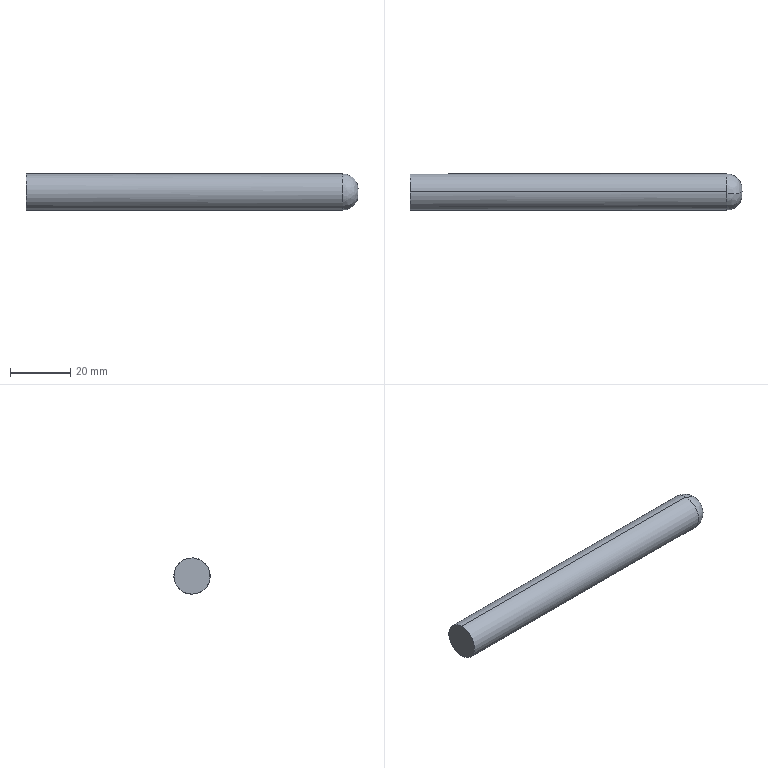Part | Creo | 1 solid | 6 faces | box 109.947 x 12 x 12 mm | volume 12270 mm3 | plane 2 | cylinder 2 | spline 2 | commonest cylinder face diameters 12 x2
STEP:
#1=CARTESIAN_POINT('',(0.,0.,0.));
#2=DIRECTION('',(0.,0.,1.));
#3=DIRECTION('',(1.,0.,0.));
#4=AXIS2_PLACEMENT_3D('',#1,#2,#3);
#5=CARTESIAN_POINT('',(51.36,96.983,-27.835));
#6=VERTEX_POINT('',#5);
#7=CARTESIAN_POINT('',(51.36,96.983,-39.835));
#8=VERTEX_POINT('',#7);
#9=CARTESIAN_POINT('',(51.36,96.983,-33.835));
#10=DIRECTION('',(-1.,0.,0.000000164));
#11=DIRECTION('',(0.000000164,0.,1.));
#12=AXIS2_PLACEMENT_3D('',#9,#10,#11);
#13=CIRCLE('',#12,6.);
#14=EDGE_CURVE('',#6,#8,#13,.T.);
#15=ORIENTED_EDGE('',*,*,#14,.F.);
#16=CARTESIAN_POINT('',(51.36,95.729,-27.968));
#17=VERTEX_POINT('',#16);
#18=CARTESIAN_POINT('',(51.36,96.983,-33.835));
#19=DIRECTION('',(-1.,0.,0.000000164));
#20=DIRECTION('',(0.000000161,-0.209,0.9779));
#21=AXIS2_PLACEMENT_3D('',#18,#19,#20);
#22=CIRCLE('',#21,6.);
#23=EDGE_CURVE('',#17,#6,#22,.T.);
#24=ORIENTED_EDGE('',*,*,#23,.F.);
#25=CARTESIAN_POINT('',(51.36,96.983,-33.835));
#26=DIRECTION('',(-1.,0.,0.000000164));
#27=DIRECTION('',(-0.000000164,0.,-1.));
#28=AXIS2_PLACEMENT_3D('',#25,#26,#27);
#29=CIRCLE('',#28,6.);
#30=EDGE_CURVE('',#8,#17,#29,.T.);
#31=ORIENTED_EDGE('',*,*,#30,.F.);
#32=EDGE_LOOP('',(#15,#24,#31));
#33=FACE_OUTER_BOUND('',#32,.F.);
#34=CARTESIAN_POINT('',(51.36,96.983,-33.835));
#35=DIRECTION('',(-1.,0.,0.000000197));
#36=DIRECTION('',(0.000000197,0.,1.));
#37=AXIS2_PLACEMENT_3D('',#34,#35,#36);
#38=PLANE('',#37);
#39=ADVANCED_FACE('',(#33),#38,.T.);
#40=CARTESIAN_POINT('',(156.307,97.613,-39.802));
#41=VERTEX_POINT('',#40);
#42=CARTESIAN_POINT('',(156.307,96.983,-27.835));
#43=VERTEX_POINT('',#42);
#44=CARTESIAN_POINT('',(156.307,96.983,-33.835));
#45=DIRECTION('',(1.,0.,-0.000000164));
#46=DIRECTION('',(-0.000000164,0.1051,-0.9945));
#47=AXIS2_PLACEMENT_3D('',#44,#45,#46);
#48=CIRCLE('',#47,6.);
#49=EDGE_CURVE('',#41,#43,#48,.T.);
#50=ORIENTED_EDGE('',*,*,#49,.T.);
#51=CARTESIAN_POINT('',(156.307,96.983,-27.835));
#52=DIRECTION('',(-1.,0.000001829,0.00000016));
#53=VECTOR('',#52,104.947);
#54=LINE('',#51,#53);
#55=EDGE_CURVE('',#43,#6,#54,.T.);
#56=ORIENTED_EDGE('',*,*,#55,.T.);
#57=ORIENTED_EDGE('',*,*,#14,.T.);
#58=CARTESIAN_POINT('',(156.307,96.983,-39.835));
#59=VERTEX_POINT('',#58);
#60=CARTESIAN_POINT('',(156.307,96.983,-39.835));
#61=DIRECTION('',(-1.,-0.000001503,0.000000164));
#62=VECTOR('',#61,104.947);
#63=LINE('',#60,#62);
#64=EDGE_CURVE('',#59,#8,#63,.T.);
#65=ORIENTED_EDGE('',*,*,#64,.F.);
#66=CARTESIAN_POINT('',(156.307,96.983,-33.835));
#67=DIRECTION('',(1.,0.,-0.000000164));
#68=DIRECTION('',(-0.000000164,0.,-1.));
#69=AXIS2_PLACEMENT_3D('',#66,#67,#68);
#70=CIRCLE('',#69,6.);
#71=EDGE_CURVE('',#59,#41,#70,.T.);
#72=ORIENTED_EDGE('',*,*,#71,.T.);
#73=EDGE_LOOP('',(#50,#56,#57,#65,#72));
#74=FACE_OUTER_BOUND('',#73,.F.);
#75=CARTESIAN_POINT('',(132.478,96.983,-33.835));
#76=DIRECTION('',(-1.,0.,0.000000164));
#77=DIRECTION('',(0.000000164,0.,1.));
#78=AXIS2_PLACEMENT_3D('',#75,#76,#77);
#79=CYLINDRICAL_SURFACE('',#78,6.);
#80=ADVANCED_FACE('',(#74),#79,.T.);
#81=ORIENTED_EDGE('',*,*,#49,.F.);
#82=CARTESIAN_POINT('',(161.307,97.088,-34.83));
#83=VERTEX_POINT('',#82);
#84=CARTESIAN_POINT('',(156.307,97.088,-34.83));
#85=DIRECTION('',(-0.000000017,-0.9945,-0.1051));
#86=DIRECTION('',(-0.000000164,0.1051,-0.9945));
#87=AXIS2_PLACEMENT_3D('',#84,#85,#86);
#88=CIRCLE('',#87,5.);
#89=EDGE_CURVE('',#41,#83,#88,.T.);
#90=ORIENTED_EDGE('',*,*,#89,.T.);
#91=CARTESIAN_POINT('',(161.307,96.878,-32.841));
#92=VERTEX_POINT('',#91);
#93=CARTESIAN_POINT('',(161.307,97.088,-34.83));
#94=CARTESIAN_POINT('',(161.307,97.197,-34.818));
#95=CARTESIAN_POINT('',(161.307,97.398,-34.763));
#96=CARTESIAN_POINT('',(161.307,97.667,-34.587));
#97=CARTESIAN_POINT('',(161.307,97.863,-34.343));
#98=CARTESIAN_POINT('',(161.307,97.977,-34.05));
#99=CARTESIAN_POINT('',(161.307,97.994,-33.732));
#100=CARTESIAN_POINT('',(161.307,97.913,-33.425));
#101=CARTESIAN_POINT('',(161.307,97.743,-33.16));
#102=CARTESIAN_POINT('',(161.307,97.499,-32.959));
#103=CARTESIAN_POINT('',(161.307,97.196,-32.841));
#104=CARTESIAN_POINT('',(161.307,96.987,-32.829));
#105=CARTESIAN_POINT('',(161.307,96.878,-32.841));
#106=B_SPLINE_CURVE_WITH_KNOTS('',3,(#93,#94,#95,#96,#97,#98,#99,#100,#101,#102,#103,#104,#105),.UNSPECIFIED.,.F.,.F.,(4,1,1,1,1,1,1,1,1,1,4),(0.,0.1,0.2,0.3,0.4,0.5,0.6,0.7,0.8,0.9,1.),.UNSPECIFIED.);
#107=EDGE_CURVE('',#83,#92,#106,.T.);
#108=ORIENTED_EDGE('',*,*,#107,.T.);
#109=CARTESIAN_POINT('',(156.307,96.353,-27.869));
#110=VERTEX_POINT('',#109);
#111=CARTESIAN_POINT('',(156.307,96.878,-32.841));
#112=DIRECTION('',(0.000000017,0.9945,0.1051));
#113=DIRECTION('',(0.000000164,-0.1051,0.9945));
#114=AXIS2_PLACEMENT_3D('',#111,#112,#113);
#115=CIRCLE('',#114,5.);
#116=EDGE_CURVE('',#110,#92,#115,.T.);
#117=ORIENTED_EDGE('',*,*,#116,.F.);
#118=CARTESIAN_POINT('',(156.307,96.983,-33.835));
#119=DIRECTION('',(1.,0.,-0.000000164));
#120=DIRECTION('',(0.000000164,0.,1.));
#121=AXIS2_PLACEMENT_3D('',#118,#119,#120);
#122=CIRCLE('',#121,6.);
#123=EDGE_CURVE('',#43,#110,#122,.T.);
#124=ORIENTED_EDGE('',*,*,#123,.F.);
#125=EDGE_LOOP('',(#81,#90,#108,#117,#124));
#126=FACE_OUTER_BOUND('',#125,.F.);
#127=CARTESIAN_POINT('',(156.15,96.813,-39.83));
#128=CARTESIAN_POINT('',(159.226,96.81,-39.927));
#129=CARTESIAN_POINT('',(161.402,96.872,-37.752));
#130=CARTESIAN_POINT('',(161.305,96.959,-34.677));
#131=CARTESIAN_POINT('',(156.15,100.709,-39.941));
#132=CARTESIAN_POINT('',(159.226,100.769,-40.039));
#133=CARTESIAN_POINT('',(161.402,99.417,-37.824));
#134=CARTESIAN_POINT('',(161.305,97.506,-34.692));
#135=CARTESIAN_POINT('',(156.15,103.357,-37.081));
#136=CARTESIAN_POINT('',(159.226,103.46,-37.133));
#137=CARTESIAN_POINT('',(161.402,101.147,-35.956));
#138=CARTESIAN_POINT('',(161.305,97.878,-34.291));
#139=CARTESIAN_POINT('',(156.15,102.947,-33.205));
#140=CARTESIAN_POINT('',(159.226,103.043,-33.195));
#141=CARTESIAN_POINT('',(161.402,100.879,-33.424));
#142=CARTESIAN_POINT('',(161.305,97.82,-33.747));
#143=CARTESIAN_POINT('',(156.15,102.538,-29.329));
#144=CARTESIAN_POINT('',(159.226,102.627,-29.256));
#145=CARTESIAN_POINT('',(161.402,100.612,-30.892));
#146=CARTESIAN_POINT('',(161.305,97.763,-33.203));
#147=CARTESIAN_POINT('',(156.15,99.351,-27.086));
#148=CARTESIAN_POINT('',(159.226,99.389,-26.977));
#149=CARTESIAN_POINT('',(161.402,98.53,-29.426));
#150=CARTESIAN_POINT('',(161.305,97.315,-32.888));
#151=CARTESIAN_POINT('',(156.15,95.564,-28.008));
#152=CARTESIAN_POINT('',(159.226,95.541,-27.914));
#153=CARTESIAN_POINT('',(161.402,96.056,-30.029));
#154=CARTESIAN_POINT('',(161.305,96.784,-33.017));
#155=(BOUNDED_SURFACE()B_SPLINE_SURFACE(3,3,((#127,#128,#129,#130),(#131,#132,#133,#134),(#135,#136,#137,#138),(#139,#140,#141,#142),(#143,#144,#145,#146),(#147,#148,#149,#150),(#151,#152,#153,#154)),.UNSPECIFIED.,.F.,.F.,.F.)B_SPLINE_SURFACE_WITH_KNOTS((4,3,4),(4,4),(0.,1.,2.),(0.,1.),.UNSPECIFIED.)GEOMETRIC_REPRESENTATION_ITEM()RATIONAL_B_SPLINE_SURFACE(((1.432,1.131,1.131,1.432),(1.106,0.8732,0.8732,1.106),(1.106,0.8732,0.8732,1.106),(1.432,1.131,1.131,1.432),(1.106,0.8732,0.8732,1.106),(1.106,0.8732,0.8732,1.106),(1.432,1.131,1.131,1.432)))REPRESENTATION_ITEM('')SURFACE());
#156=ADVANCED_FACE('',(#126),#155,.T.);
#157=CARTESIAN_POINT('',(156.307,96.983,-33.835));
#158=DIRECTION('',(1.,0.,-0.000000164));
#159=DIRECTION('',(0.000000164,-0.1051,0.9945));
#160=AXIS2_PLACEMENT_3D('',#157,#158,#159);
#161=CIRCLE('',#160,6.);
#162=EDGE_CURVE('',#110,#59,#161,.T.);
#163=ORIENTED_EDGE('',*,*,#162,.F.);
#164=ORIENTED_EDGE('',*,*,#116,.T.);
#165=CARTESIAN_POINT('',(161.307,96.878,-32.841));
#166=CARTESIAN_POINT('',(161.307,96.769,-32.852));
#167=CARTESIAN_POINT('',(161.307,96.568,-32.908));
#168=CARTESIAN_POINT('',(161.307,96.299,-33.083));
#169=CARTESIAN_POINT('',(161.307,96.103,-33.327));
#170=CARTESIAN_POINT('',(161.307,95.99,-33.621));
#171=CARTESIAN_POINT('',(161.307,95.972,-33.938));
#172=CARTESIAN_POINT('',(161.307,96.053,-34.245));
#173=CARTESIAN_POINT('',(161.307,96.224,-34.51));
#174=CARTESIAN_POINT('',(161.307,96.467,-34.712));
#175=CARTESIAN_POINT('',(161.307,96.77,-34.829));
#176=CARTESIAN_POINT('',(161.307,96.979,-34.841));
#177=CARTESIAN_POINT('',(161.307,97.088,-34.83));
#178=B_SPLINE_CURVE_WITH_KNOTS('',3,(#165,#166,#167,#168,#169,#170,#171,#172,#173,#174,#175,#176,#177),.UNSPECIFIED.,.F.,.F.,(4,1,1,1,1,1,1,1,1,1,4),(0.,0.1,0.2,0.3,0.4,0.5,0.6,0.7,0.8,0.9,1.),.UNSPECIFIED.);
#179=EDGE_CURVE('',#92,#83,#178,.T.);
#180=ORIENTED_EDGE('',*,*,#179,.T.);
#181=ORIENTED_EDGE('',*,*,#89,.F.);
#182=ORIENTED_EDGE('',*,*,#71,.F.);
#183=EDGE_LOOP('',(#163,#164,#180,#181,#182));
#184=FACE_OUTER_BOUND('',#183,.F.);
#185=CARTESIAN_POINT('',(156.15,97.153,-27.84));
#186=CARTESIAN_POINT('',(159.226,97.156,-27.744));
#187=CARTESIAN_POINT('',(161.402,97.094,-29.919));
#188=CARTESIAN_POINT('',(161.305,97.007,-32.994));
#189=CARTESIAN_POINT('',(156.15,93.257,-27.73));
#190=CARTESIAN_POINT('',(159.226,93.197,-27.631));
#191=CARTESIAN_POINT('',(161.402,94.549,-29.847));
#192=CARTESIAN_POINT('',(161.305,96.46,-32.978));
#193=CARTESIAN_POINT('',(156.15,90.609,-30.59));
#194=CARTESIAN_POINT('',(159.226,90.506,-30.537));
#195=CARTESIAN_POINT('',(161.402,92.819,-31.715));
#196=CARTESIAN_POINT('',(161.305,96.088,-33.38));
#197=CARTESIAN_POINT('',(156.15,91.019,-34.466));
#198=CARTESIAN_POINT('',(159.226,90.923,-34.476));
#199=CARTESIAN_POINT('',(161.402,93.087,-34.247));
#200=CARTESIAN_POINT('',(161.305,96.146,-33.924));
#201=CARTESIAN_POINT('',(156.15,91.428,-38.342));
#202=CARTESIAN_POINT('',(159.226,91.339,-38.414));
#203=CARTESIAN_POINT('',(161.402,93.354,-36.779));
#204=CARTESIAN_POINT('',(161.305,96.203,-34.468));
#205=CARTESIAN_POINT('',(156.15,94.615,-40.585));
#206=CARTESIAN_POINT('',(159.226,94.577,-40.694));
#207=CARTESIAN_POINT('',(161.402,95.436,-38.244));
#208=CARTESIAN_POINT('',(161.305,96.651,-34.783));
#209=CARTESIAN_POINT('',(156.15,98.402,-39.663));
#210=CARTESIAN_POINT('',(159.226,98.425,-39.756));
#211=CARTESIAN_POINT('',(161.402,97.91,-37.642));
#212=CARTESIAN_POINT('',(161.305,97.182,-34.653));
#213=(BOUNDED_SURFACE()B_SPLINE_SURFACE(3,3,((#185,#186,#187,#188),(#189,#190,#191,#192),(#193,#194,#195,#196),(#197,#198,#199,#200),(#201,#202,#203,#204),(#205,#206,#207,#208),(#209,#210,#211,#212)),.UNSPECIFIED.,.F.,.F.,.F.)B_SPLINE_SURFACE_WITH_KNOTS((4,3,4),(4,4),(0.,1.,2.),(0.,1.),.UNSPECIFIED.)GEOMETRIC_REPRESENTATION_ITEM()RATIONAL_B_SPLINE_SURFACE(((1.432,1.131,1.131,1.432),(1.106,0.8732,0.8732,1.106),(1.106,0.8732,0.8732,1.106),(1.432,1.131,1.131,1.432),(1.106,0.8732,0.8732,1.106),(1.106,0.8732,0.8732,1.106),(1.432,1.131,1.131,1.432)))REPRESENTATION_ITEM('')SURFACE());
#214=ADVANCED_FACE('',(#184),#213,.T.);
#215=ORIENTED_EDGE('',*,*,#123,.T.);
#216=ORIENTED_EDGE('',*,*,#162,.T.);
#217=ORIENTED_EDGE('',*,*,#64,.T.);
#218=ORIENTED_EDGE('',*,*,#30,.T.);
#219=ORIENTED_EDGE('',*,*,#23,.T.);
#220=ORIENTED_EDGE('',*,*,#55,.F.);
#221=EDGE_LOOP('',(#215,#216,#217,#218,#219,#220));
#222=FACE_OUTER_BOUND('',#221,.F.);
#223=CARTESIAN_POINT('',(132.478,96.983,-33.835));
#224=DIRECTION('',(-1.,0.,0.000000164));
#225=DIRECTION('',(0.000000164,0.,1.));
#226=AXIS2_PLACEMENT_3D('',#223,#224,#225);
#227=CYLINDRICAL_SURFACE('',#226,6.);
#228=ADVANCED_FACE('',(#222),#227,.T.);
#229=ORIENTED_EDGE('',*,*,#179,.F.);
#230=ORIENTED_EDGE('',*,*,#107,.F.);
#231=EDGE_LOOP('',(#229,#230));
#232=FACE_OUTER_BOUND('',#231,.F.);
#233=CARTESIAN_POINT('',(161.307,96.983,-33.835));
#234=DIRECTION('',(1.,0.,-0.000000164));
#235=DIRECTION('',(-0.000000164,0.,-1.));
#236=AXIS2_PLACEMENT_3D('',#233,#234,#235);
#237=PLANE('',#236);
#238=ADVANCED_FACE('',(#232),#237,.T.);
#239=CLOSED_SHELL('',(#39,#80,#156,#214,#228,#238));
#240=MANIFOLD_SOLID_BREP('',#239);
#241=(LENGTH_UNIT()NAMED_UNIT(*)SI_UNIT(.MILLI.,.METRE.));
#242=UNCERTAINTY_MEASURE_WITH_UNIT(LENGTH_MEASURE(0.01112),#241,'','');
#243=(NAMED_UNIT(*)PLANE_ANGLE_UNIT()SI_UNIT($,.RADIAN.));
#244=PLANE_ANGLE_MEASURE_WITH_UNIT(PLANE_ANGLE_MEASURE(0.01745),#243);
#245=(CONVERSION_BASED_UNIT('DEGREE',#244)NAMED_UNIT(*)PLANE_ANGLE_UNIT());
#246=(NAMED_UNIT(*)SI_UNIT($,.STERADIAN.)SOLID_ANGLE_UNIT());
#247=(GEOMETRIC_REPRESENTATION_CONTEXT(3)GLOBAL_UNCERTAINTY_ASSIGNED_CONTEXT((#242))GLOBAL_UNIT_ASSIGNED_CONTEXT((#241,#245,#246))REPRESENTATION_CONTEXT('',''));
#248=ADVANCED_BREP_SHAPE_REPRESENTATION('',(#4,#240),#247);